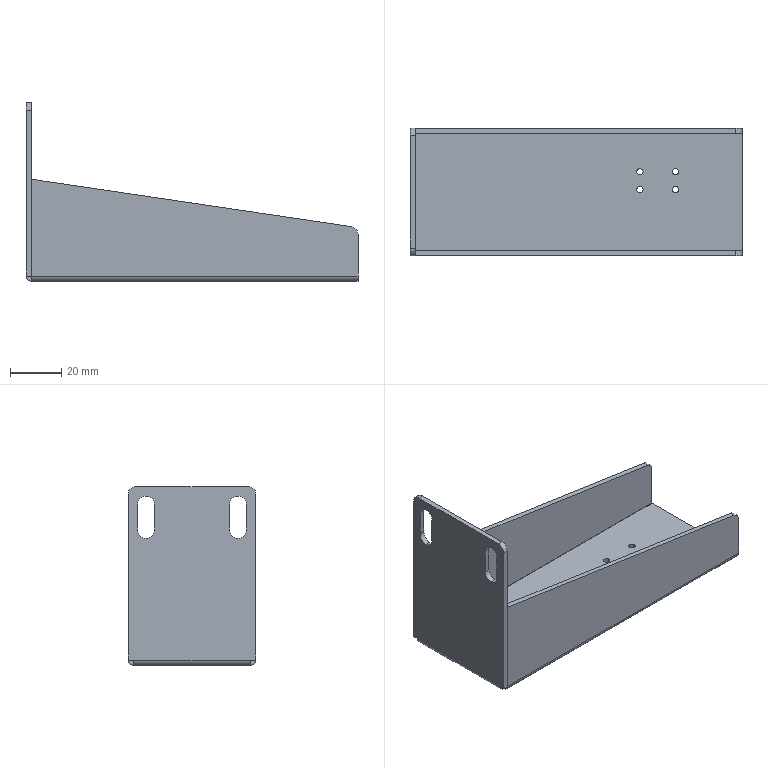Part | STEP file | 1 solid | 54 faces | box 130 x 50 x 70 mm | volume 33645 mm3 | plane 30 | cylinder 24 | commonest cylinder face diameters 2.5 x8 6.5 x6 6 x4 0.2 x3 4.2 x3